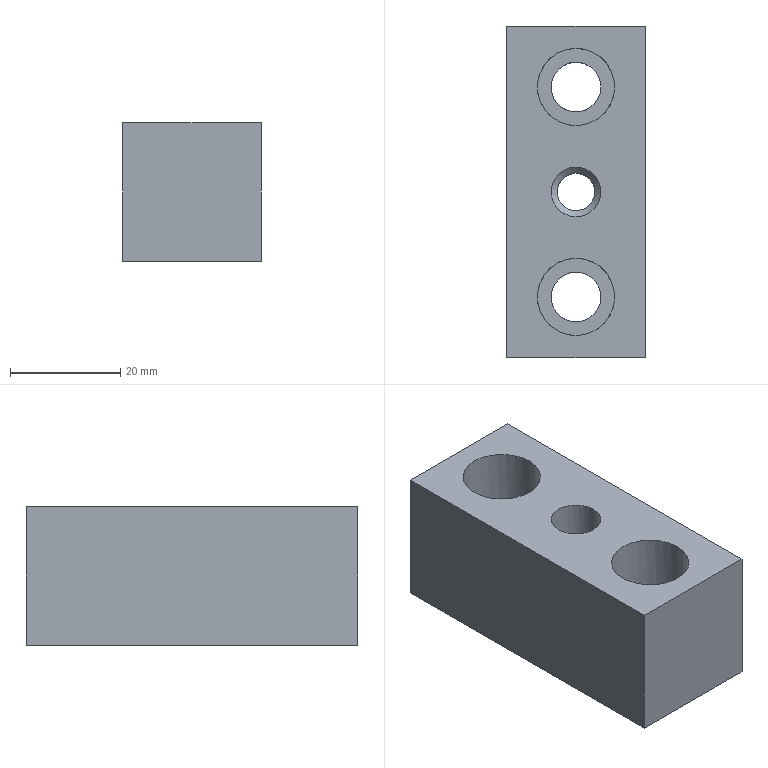Part | STEP file | gslz 2016.10.28-6_id6_x_t | 1 solid | 15 faces | box 25 x 60 x 25 mm | volume 30776 mm3 | plane 8 | cylinder 6 | cone 1 | commonest cylinder face diameters 9 x3 14 x2 6.8 x1
STEP:
#1=CARTESIAN_POINT('',(202.2,154.5,3.));
#2=VERTEX_POINT('',#1);
#3=CARTESIAN_POINT('',(202.2,150.,3.));
#4=DIRECTION('',(0.,0.,1.));
#5=DIRECTION('',(0.,1.,0.));
#6=AXIS2_PLACEMENT_3D('',#3,#4,#5);
#7=CIRCLE('',#6,4.5);
#8=EDGE_CURVE('',#2,#2,#7,.T.);
#9=ORIENTED_EDGE('',*,*,#8,.T.);
#10=EDGE_LOOP('',(#9));
#11=FACE_BOUND('',#10,.T.);
#12=CARTESIAN_POINT('',(202.2,153.4,1.9));
#13=VERTEX_POINT('',#12);
#14=CARTESIAN_POINT('',(202.2,150.,1.9));
#15=DIRECTION('',(0.,0.,1.));
#16=DIRECTION('',(0.,1.,0.));
#17=AXIS2_PLACEMENT_3D('',#14,#15,#16);
#18=CIRCLE('',#17,3.4);
#19=EDGE_CURVE('',#13,#13,#18,.T.);
#20=ORIENTED_EDGE('',*,*,#19,.F.);
#21=EDGE_LOOP('',(#20));
#22=FACE_BOUND('',#21,.T.);
#23=CARTESIAN_POINT('',(202.2,150.,1.));
#24=DIRECTION('',(0.,0.,1.));
#25=DIRECTION('',(0.,1.,0.));
#26=AXIS2_PLACEMENT_3D('',#23,#24,#25);
#27=CONICAL_SURFACE('',#26,2.5,45.);
#28=ADVANCED_FACE('',(#11,#22),#27,.F.);
#29=CARTESIAN_POINT('',(202.2,135.5,0.));
#30=VERTEX_POINT('',#29);
#31=CARTESIAN_POINT('',(202.2,131.,0.));
#32=DIRECTION('',(0.,0.,1.));
#33=DIRECTION('',(0.,1.,0.));
#34=AXIS2_PLACEMENT_3D('',#31,#32,#33);
#35=CIRCLE('',#34,4.5);
#36=EDGE_CURVE('',#30,#30,#35,.T.);
#37=ORIENTED_EDGE('',*,*,#36,.F.);
#38=EDGE_LOOP('',(#37));
#39=FACE_BOUND('',#38,.T.);
#40=CARTESIAN_POINT('',(202.2,138.,0.));
#41=VERTEX_POINT('',#40);
#42=CARTESIAN_POINT('',(202.2,131.,0.));
#43=DIRECTION('',(0.,0.,1.));
#44=DIRECTION('',(0.,1.,0.));
#45=AXIS2_PLACEMENT_3D('',#42,#43,#44);
#46=CIRCLE('',#45,7.);
#47=EDGE_CURVE('',#41,#41,#46,.T.);
#48=ORIENTED_EDGE('',*,*,#47,.T.);
#49=EDGE_LOOP('',(#48));
#50=FACE_BOUND('',#49,.T.);
#51=CARTESIAN_POINT('',(202.2,131.,0.));
#52=DIRECTION('',(0.,0.,1.));
#53=DIRECTION('',(0.,1.,0.));
#54=AXIS2_PLACEMENT_3D('',#51,#52,#53);
#55=PLANE('',#54);
#56=ADVANCED_FACE('',(#39,#50),#55,.T.);
#57=ORIENTED_EDGE('',*,*,#19,.T.);
#58=EDGE_LOOP('',(#57));
#59=FACE_BOUND('',#58,.T.);
#60=CARTESIAN_POINT('',(205.6,150.,-12.));
#61=VERTEX_POINT('',#60);
#62=CARTESIAN_POINT('',(202.2,150.,-12.));
#63=DIRECTION('',(0.,0.,-1.));
#64=DIRECTION('',(1.,0.,0.));
#65=AXIS2_PLACEMENT_3D('',#62,#63,#64);
#66=CIRCLE('',#65,3.4);
#67=EDGE_CURVE('',#61,#61,#66,.T.);
#68=ORIENTED_EDGE('',*,*,#67,.T.);
#69=EDGE_LOOP('',(#68));
#70=FACE_BOUND('',#69,.T.);
#71=CARTESIAN_POINT('',(202.2,150.,22.));
#72=DIRECTION('',(0.,0.,-1.));
#73=DIRECTION('',(0.,-1.,0.));
#74=AXIS2_PLACEMENT_3D('',#71,#72,#73);
#75=CYLINDRICAL_SURFACE('',#74,3.4);
#76=ADVANCED_FACE('',(#59,#70),#75,.F.);
#77=CARTESIAN_POINT('',(214.7,180.,13.));
#78=VERTEX_POINT('',#77);
#79=CARTESIAN_POINT('',(189.7,180.,13.));
#80=VERTEX_POINT('',#79);
#81=CARTESIAN_POINT('',(210.2,180.,13.));
#82=DIRECTION('',(-1.,0.,0.));
#83=VECTOR('',#82,1.);
#84=LINE('',#81,#83);
#85=EDGE_CURVE('',#78,#80,#84,.T.);
#86=ORIENTED_EDGE('',*,*,#85,.F.);
#87=CARTESIAN_POINT('',(214.7,180.,-12.));
#88=VERTEX_POINT('',#87);
#89=CARTESIAN_POINT('',(214.7,180.,6.));
#90=DIRECTION('',(0.,0.,1.));
#91=VECTOR('',#90,1.);
#92=LINE('',#89,#91);
#93=EDGE_CURVE('',#88,#78,#92,.T.);
#94=ORIENTED_EDGE('',*,*,#93,.F.);
#95=CARTESIAN_POINT('',(189.7,180.,-12.));
#96=VERTEX_POINT('',#95);
#97=CARTESIAN_POINT('',(210.2,180.,-12.));
#98=DIRECTION('',(-1.,0.,0.));
#99=VECTOR('',#98,1.);
#100=LINE('',#97,#99);
#101=EDGE_CURVE('',#88,#96,#100,.T.);
#102=ORIENTED_EDGE('',*,*,#101,.T.);
#103=CARTESIAN_POINT('',(189.7,180.,6.));
#104=DIRECTION('',(0.,0.,1.));
#105=VECTOR('',#104,1.);
#106=LINE('',#103,#105);
#107=EDGE_CURVE('',#96,#80,#106,.T.);
#108=ORIENTED_EDGE('',*,*,#107,.T.);
#109=EDGE_LOOP('',(#86,#94,#102,#108));
#110=FACE_OUTER_BOUND('',#109,.T.);
#111=CARTESIAN_POINT('',(210.2,180.,6.));
#112=DIRECTION('',(0.,-1.,0.));
#113=DIRECTION('',(0.,0.,1.));
#114=AXIS2_PLACEMENT_3D('',#111,#112,#113);
#115=PLANE('',#114);
#116=ADVANCED_FACE('',(#110),#115,.F.);
#117=CARTESIAN_POINT('',(189.7,120.,13.));
#118=VERTEX_POINT('',#117);
#119=CARTESIAN_POINT('',(189.7,160.,13.));
#120=DIRECTION('',(0.,-1.,0.));
#121=VECTOR('',#120,1.);
#122=LINE('',#119,#121);
#123=EDGE_CURVE('',#80,#118,#122,.T.);
#124=ORIENTED_EDGE('',*,*,#123,.F.);
#125=ORIENTED_EDGE('',*,*,#107,.F.);
#126=CARTESIAN_POINT('',(189.7,120.,-12.));
#127=VERTEX_POINT('',#126);
#128=CARTESIAN_POINT('',(189.7,160.,-12.));
#129=DIRECTION('',(0.,-1.,0.));
#130=VECTOR('',#129,1.);
#131=LINE('',#128,#130);
#132=EDGE_CURVE('',#96,#127,#131,.T.);
#133=ORIENTED_EDGE('',*,*,#132,.T.);
#134=CARTESIAN_POINT('',(189.7,120.,6.));
#135=DIRECTION('',(0.,0.,1.));
#136=VECTOR('',#135,1.);
#137=LINE('',#134,#136);
#138=EDGE_CURVE('',#127,#118,#137,.T.);
#139=ORIENTED_EDGE('',*,*,#138,.T.);
#140=EDGE_LOOP('',(#124,#125,#133,#139));
#141=FACE_OUTER_BOUND('',#140,.T.);
#142=CARTESIAN_POINT('',(189.7,160.,6.));
#143=DIRECTION('',(1.,0.,0.));
#144=DIRECTION('',(0.,0.,-1.));
#145=AXIS2_PLACEMENT_3D('',#142,#143,#144);
#146=PLANE('',#145);
#147=ADVANCED_FACE('',(#141),#146,.F.);
#148=CARTESIAN_POINT('',(214.7,120.,-12.));
#149=VERTEX_POINT('',#148);
#150=CARTESIAN_POINT('',(194.2,120.,-12.));
#151=DIRECTION('',(1.,0.,0.));
#152=VECTOR('',#151,1.);
#153=LINE('',#150,#152);
#154=EDGE_CURVE('',#127,#149,#153,.T.);
#155=ORIENTED_EDGE('',*,*,#154,.T.);
#156=CARTESIAN_POINT('',(214.7,120.,13.));
#157=VERTEX_POINT('',#156);
#158=CARTESIAN_POINT('',(214.7,120.,6.));
#159=DIRECTION('',(0.,0.,1.));
#160=VECTOR('',#159,1.);
#161=LINE('',#158,#160);
#162=EDGE_CURVE('',#149,#157,#161,.T.);
#163=ORIENTED_EDGE('',*,*,#162,.T.);
#164=CARTESIAN_POINT('',(194.2,120.,13.));
#165=DIRECTION('',(1.,0.,0.));
#166=VECTOR('',#165,1.);
#167=LINE('',#164,#166);
#168=EDGE_CURVE('',#118,#157,#167,.T.);
#169=ORIENTED_EDGE('',*,*,#168,.F.);
#170=ORIENTED_EDGE('',*,*,#138,.F.);
#171=EDGE_LOOP('',(#155,#163,#169,#170));
#172=FACE_OUTER_BOUND('',#171,.T.);
#173=CARTESIAN_POINT('',(194.2,120.,6.));
#174=DIRECTION('',(0.,1.,0.));
#175=DIRECTION('',(0.,0.,-1.));
#176=AXIS2_PLACEMENT_3D('',#173,#174,#175);
#177=PLANE('',#176);
#178=ADVANCED_FACE('',(#172),#177,.F.);
#179=CARTESIAN_POINT('',(214.7,130.,13.));
#180=DIRECTION('',(0.,1.,0.));
#181=VECTOR('',#180,1.);
#182=LINE('',#179,#181);
#183=EDGE_CURVE('',#157,#78,#182,.T.);
#184=ORIENTED_EDGE('',*,*,#183,.F.);
#185=ORIENTED_EDGE('',*,*,#162,.F.);
#186=CARTESIAN_POINT('',(214.7,130.,-12.));
#187=DIRECTION('',(0.,1.,0.));
#188=VECTOR('',#187,1.);
#189=LINE('',#186,#188);
#190=EDGE_CURVE('',#149,#88,#189,.T.);
#191=ORIENTED_EDGE('',*,*,#190,.T.);
#192=ORIENTED_EDGE('',*,*,#93,.T.);
#193=EDGE_LOOP('',(#184,#185,#191,#192));
#194=FACE_OUTER_BOUND('',#193,.T.);
#195=CARTESIAN_POINT('',(214.7,130.,6.));
#196=DIRECTION('',(-1.,0.,0.));
#197=DIRECTION('',(0.,0.,1.));
#198=AXIS2_PLACEMENT_3D('',#195,#196,#197);
#199=PLANE('',#198);
#200=ADVANCED_FACE('',(#194),#199,.F.);
#201=CARTESIAN_POINT('',(206.7,131.,-12.));
#202=VERTEX_POINT('',#201);
#203=CARTESIAN_POINT('',(202.2,131.,-12.));
#204=DIRECTION('',(0.,0.,-1.));
#205=DIRECTION('',(1.,0.,0.));
#206=AXIS2_PLACEMENT_3D('',#203,#204,#205);
#207=CIRCLE('',#206,4.5);
#208=EDGE_CURVE('',#202,#202,#207,.T.);
#209=ORIENTED_EDGE('',*,*,#208,.T.);
#210=EDGE_LOOP('',(#209));
#211=FACE_BOUND('',#210,.T.);
#212=ORIENTED_EDGE('',*,*,#36,.T.);
#213=EDGE_LOOP('',(#212));
#214=FACE_BOUND('',#213,.T.);
#215=CARTESIAN_POINT('',(202.2,131.,22.));
#216=DIRECTION('',(0.,0.,-1.));
#217=DIRECTION('',(0.,-1.,0.));
#218=AXIS2_PLACEMENT_3D('',#215,#216,#217);
#219=CYLINDRICAL_SURFACE('',#218,4.5);
#220=ADVANCED_FACE('',(#211,#214),#219,.F.);
#221=ORIENTED_EDGE('',*,*,#208,.F.);
#222=EDGE_LOOP('',(#221));
#223=FACE_BOUND('',#222,.T.);
#224=ORIENTED_EDGE('',*,*,#190,.F.);
#225=ORIENTED_EDGE('',*,*,#154,.F.);
#226=ORIENTED_EDGE('',*,*,#132,.F.);
#227=ORIENTED_EDGE('',*,*,#101,.F.);
#228=EDGE_LOOP('',(#224,#225,#226,#227));
#229=FACE_BOUND('',#228,.T.);
#230=ORIENTED_EDGE('',*,*,#67,.F.);
#231=EDGE_LOOP('',(#230));
#232=FACE_BOUND('',#231,.T.);
#233=CARTESIAN_POINT('',(206.7,169.,-12.));
#234=VERTEX_POINT('',#233);
#235=CARTESIAN_POINT('',(202.2,169.,-12.));
#236=DIRECTION('',(0.,0.,-1.));
#237=DIRECTION('',(1.,0.,0.));
#238=AXIS2_PLACEMENT_3D('',#235,#236,#237);
#239=CIRCLE('',#238,4.5);
#240=EDGE_CURVE('',#234,#234,#239,.T.);
#241=ORIENTED_EDGE('',*,*,#240,.F.);
#242=EDGE_LOOP('',(#241));
#243=FACE_BOUND('',#242,.T.);
#244=CARTESIAN_POINT('',(-210.2,130.,-12.));
#245=DIRECTION('',(0.,0.,1.));
#246=DIRECTION('',(0.,1.,0.));
#247=AXIS2_PLACEMENT_3D('',#244,#245,#246);
#248=PLANE('',#247);
#249=ADVANCED_FACE('',(#223,#229,#232,#243),#248,.F.);
#250=ORIENTED_EDGE('',*,*,#47,.F.);
#251=EDGE_LOOP('',(#250));
#252=FACE_BOUND('',#251,.T.);
#253=CARTESIAN_POINT('',(209.2,131.,13.));
#254=VERTEX_POINT('',#253);
#255=CARTESIAN_POINT('',(202.2,131.,13.));
#256=DIRECTION('',(0.,0.,1.));
#257=DIRECTION('',(1.,0.,0.));
#258=AXIS2_PLACEMENT_3D('',#255,#256,#257);
#259=CIRCLE('',#258,7.);
#260=EDGE_CURVE('',#254,#254,#259,.T.);
#261=ORIENTED_EDGE('',*,*,#260,.T.);
#262=EDGE_LOOP('',(#261));
#263=FACE_BOUND('',#262,.T.);
#264=CARTESIAN_POINT('',(202.2,131.,-2.));
#265=DIRECTION('',(0.,0.,1.));
#266=DIRECTION('',(0.,1.,0.));
#267=AXIS2_PLACEMENT_3D('',#264,#265,#266);
#268=CYLINDRICAL_SURFACE('',#267,7.);
#269=ADVANCED_FACE('',(#252,#263),#268,.F.);
#270=ORIENTED_EDGE('',*,*,#8,.F.);
#271=EDGE_LOOP('',(#270));
#272=FACE_BOUND('',#271,.T.);
#273=CARTESIAN_POINT('',(206.7,150.,13.));
#274=VERTEX_POINT('',#273);
#275=CARTESIAN_POINT('',(202.2,150.,13.));
#276=DIRECTION('',(0.,0.,1.));
#277=DIRECTION('',(1.,0.,0.));
#278=AXIS2_PLACEMENT_3D('',#275,#276,#277);
#279=CIRCLE('',#278,4.5);
#280=EDGE_CURVE('',#274,#274,#279,.T.);
#281=ORIENTED_EDGE('',*,*,#280,.T.);
#282=EDGE_LOOP('',(#281));
#283=FACE_BOUND('',#282,.T.);
#284=CARTESIAN_POINT('',(202.2,150.,-2.));
#285=DIRECTION('',(0.,0.,1.));
#286=DIRECTION('',(0.,1.,0.));
#287=AXIS2_PLACEMENT_3D('',#284,#285,#286);
#288=CYLINDRICAL_SURFACE('',#287,4.5);
#289=ADVANCED_FACE('',(#272,#283),#288,.F.);
#290=CARTESIAN_POINT('',(209.2,169.,13.));
#291=VERTEX_POINT('',#290);
#292=CARTESIAN_POINT('',(202.2,169.,13.));
#293=DIRECTION('',(0.,0.,1.));
#294=DIRECTION('',(1.,0.,0.));
#295=AXIS2_PLACEMENT_3D('',#292,#293,#294);
#296=CIRCLE('',#295,7.);
#297=EDGE_CURVE('',#291,#291,#296,.T.);
#298=ORIENTED_EDGE('',*,*,#297,.F.);
#299=EDGE_LOOP('',(#298));
#300=FACE_BOUND('',#299,.T.);
#301=ORIENTED_EDGE('',*,*,#280,.F.);
#302=EDGE_LOOP('',(#301));
#303=FACE_BOUND('',#302,.T.);
#304=ORIENTED_EDGE('',*,*,#260,.F.);
#305=EDGE_LOOP('',(#304));
#306=FACE_BOUND('',#305,.T.);
#307=ORIENTED_EDGE('',*,*,#168,.T.);
#308=ORIENTED_EDGE('',*,*,#183,.T.);
#309=ORIENTED_EDGE('',*,*,#85,.T.);
#310=ORIENTED_EDGE('',*,*,#123,.T.);
#311=EDGE_LOOP('',(#307,#308,#309,#310));
#312=FACE_BOUND('',#311,.T.);
#313=CARTESIAN_POINT('',(-210.2,130.,13.));
#314=DIRECTION('',(0.,0.,1.));
#315=DIRECTION('',(0.,1.,0.));
#316=AXIS2_PLACEMENT_3D('',#313,#314,#315);
#317=PLANE('',#316);
#318=ADVANCED_FACE('',(#300,#303,#306,#312),#317,.T.);
#319=CARTESIAN_POINT('',(202.2,173.5,0.));
#320=VERTEX_POINT('',#319);
#321=CARTESIAN_POINT('',(202.2,169.,0.));
#322=DIRECTION('',(0.,0.,1.));
#323=DIRECTION('',(0.,1.,0.));
#324=AXIS2_PLACEMENT_3D('',#321,#322,#323);
#325=CIRCLE('',#324,4.5);
#326=EDGE_CURVE('',#320,#320,#325,.T.);
#327=ORIENTED_EDGE('',*,*,#326,.F.);
#328=EDGE_LOOP('',(#327));
#329=FACE_BOUND('',#328,.T.);
#330=CARTESIAN_POINT('',(202.2,176.,0.));
#331=VERTEX_POINT('',#330);
#332=CARTESIAN_POINT('',(202.2,169.,0.));
#333=DIRECTION('',(0.,0.,1.));
#334=DIRECTION('',(0.,1.,0.));
#335=AXIS2_PLACEMENT_3D('',#332,#333,#334);
#336=CIRCLE('',#335,7.);
#337=EDGE_CURVE('',#331,#331,#336,.T.);
#338=ORIENTED_EDGE('',*,*,#337,.T.);
#339=EDGE_LOOP('',(#338));
#340=FACE_BOUND('',#339,.T.);
#341=CARTESIAN_POINT('',(202.2,169.,0.));
#342=DIRECTION('',(0.,0.,1.));
#343=DIRECTION('',(0.,1.,0.));
#344=AXIS2_PLACEMENT_3D('',#341,#342,#343);
#345=PLANE('',#344);
#346=ADVANCED_FACE('',(#329,#340),#345,.T.);
#347=ORIENTED_EDGE('',*,*,#240,.T.);
#348=EDGE_LOOP('',(#347));
#349=FACE_BOUND('',#348,.T.);
#350=ORIENTED_EDGE('',*,*,#326,.T.);
#351=EDGE_LOOP('',(#350));
#352=FACE_BOUND('',#351,.T.);
#353=CARTESIAN_POINT('',(202.2,169.,22.));
#354=DIRECTION('',(0.,0.,-1.));
#355=DIRECTION('',(0.,-1.,0.));
#356=AXIS2_PLACEMENT_3D('',#353,#354,#355);
#357=CYLINDRICAL_SURFACE('',#356,4.5);
#358=ADVANCED_FACE('',(#349,#352),#357,.F.);
#359=ORIENTED_EDGE('',*,*,#337,.F.);
#360=EDGE_LOOP('',(#359));
#361=FACE_BOUND('',#360,.T.);
#362=ORIENTED_EDGE('',*,*,#297,.T.);
#363=EDGE_LOOP('',(#362));
#364=FACE_BOUND('',#363,.T.);
#365=CARTESIAN_POINT('',(202.2,169.,-2.));
#366=DIRECTION('',(0.,0.,1.));
#367=DIRECTION('',(0.,1.,0.));
#368=AXIS2_PLACEMENT_3D('',#365,#366,#367);
#369=CYLINDRICAL_SURFACE('',#368,7.);
#370=ADVANCED_FACE('',(#361,#364),#369,.F.);
#371=CLOSED_SHELL('',(#28,#56,#76,#116,#147,#178,#200,#220,#249,#269,#289,#318,#346,#358,#370));
#372=MANIFOLD_SOLID_BREP('',#371);
#373=(LENGTH_UNIT()NAMED_UNIT(*)SI_UNIT(.MILLI.,.METRE.));
#374=UNCERTAINTY_MEASURE_WITH_UNIT(LENGTH_MEASURE(0.00002),#373,'','');
#375=(NAMED_UNIT(*)PLANE_ANGLE_UNIT()SI_UNIT($,.RADIAN.));
#376=PLANE_ANGLE_MEASURE_WITH_UNIT(PLANE_ANGLE_MEASURE(0.01745),#375);
#377=DIMENSIONAL_EXPONENTS(0.,0.,0.,0.,0.,0.,0.);
#378=(CONVERSION_BASED_UNIT('DEGREE',#376)NAMED_UNIT(#377)PLANE_ANGLE_UNIT());
#379=(NAMED_UNIT(*)SI_UNIT($,.STERADIAN.)SOLID_ANGLE_UNIT());
#380=(GEOMETRIC_REPRESENTATION_CONTEXT(3)GLOBAL_UNCERTAINTY_ASSIGNED_CONTEXT((#374))GLOBAL_UNIT_ASSIGNED_CONTEXT((#373,#378,#379))REPRESENTATION_CONTEXT('',''));
#381=ADVANCED_BREP_SHAPE_REPRESENTATION('',(#372),#380);